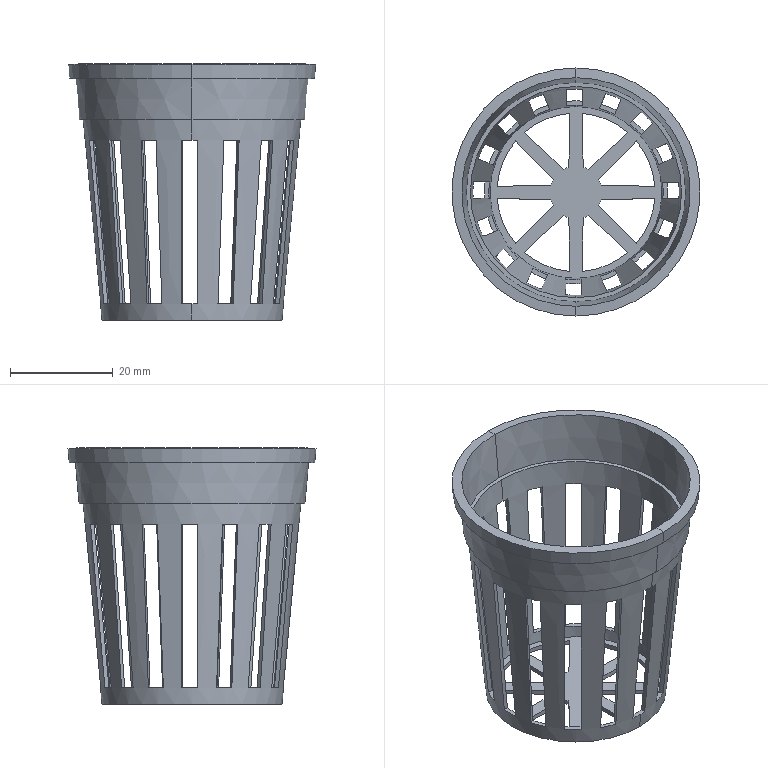Part | SolidWorks | features BaseBody 1 | 1 solid | 113 faces | box 48.245 x 48.245 x 49.817 mm | volume 4404 mm3 | plane 85 | cylinder 16 | cone 12 | commonest cylinder face diameters 10.222 x8 30.787 x8